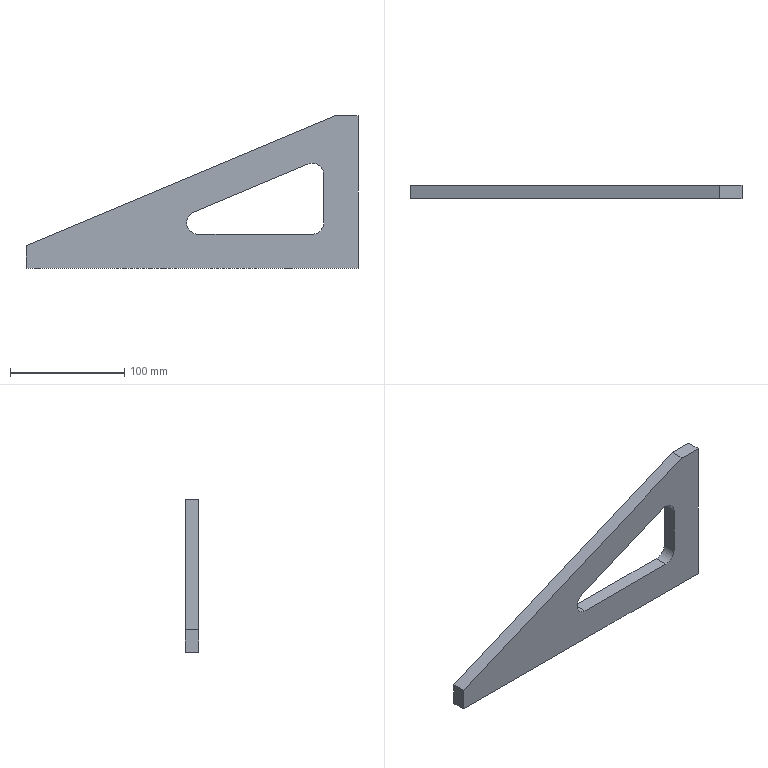Part | SolidWorks | features HoleWzd 2, Extrusion 1, ICE 1 | 1 solid | 34 faces | box 291 x 12 x 134 mm | volume 221726 mm3 | cylinder 14 | cone 10 | plane 10 | commonest cylinder face diameters 5 x10 20 x4
STEP:
#1=CARTESIAN_POINT('',(-133.,0.,-52.));
#2=VERTEX_POINT('',#1);
#3=CARTESIAN_POINT('',(-138.,0.,-52.));
#4=VERTEX_POINT('',#3);
#5=CARTESIAN_POINT('',(-135.5,0.,-52.));
#6=DIRECTION('',(0.,0.,-1.));
#7=DIRECTION('',(-1.,0.,0.));
#8=AXIS2_PLACEMENT_3D('',#5,#6,#7);
#9=CIRCLE('',#8,2.5);
#10=EDGE_CURVE('',#2,#4,#9,.T.);
#11=ORIENTED_EDGE('',*,*,#10,.F.);
#12=CARTESIAN_POINT('',(-133.,0.,-67.));
#13=VERTEX_POINT('',#12);
#14=CARTESIAN_POINT('',(-133.,0.,-67.));
#15=DIRECTION('',(0.,0.,-1.));
#16=VECTOR('',#15,1000.);
#17=LINE('',#14,#16);
#18=EDGE_CURVE('',#2,#13,#17,.T.);
#19=ORIENTED_EDGE('',*,*,#18,.T.);
#20=CARTESIAN_POINT('',(-138.,0.,-67.));
#21=VERTEX_POINT('',#20);
#22=CARTESIAN_POINT('',(-135.5,0.,-67.));
#23=DIRECTION('',(0.,0.,-1.));
#24=DIRECTION('',(-1.,0.,0.));
#25=AXIS2_PLACEMENT_3D('',#22,#23,#24);
#26=CIRCLE('',#25,2.5);
#27=EDGE_CURVE('',#13,#21,#26,.T.);
#28=ORIENTED_EDGE('',*,*,#27,.T.);
#29=CARTESIAN_POINT('',(-138.,0.,-67.));
#30=DIRECTION('',(0.,0.,-1.));
#31=VECTOR('',#30,1000.);
#32=LINE('',#29,#31);
#33=EDGE_CURVE('',#4,#21,#32,.T.);
#34=ORIENTED_EDGE('',*,*,#33,.F.);
#35=EDGE_LOOP('',(#11,#19,#28,#34));
#36=FACE_OUTER_BOUND('',#35,.T.);
#37=CARTESIAN_POINT('',(-135.5,0.,-67.));
#38=DIRECTION('',(0.,0.,-1.));
#39=DIRECTION('',(-1.,0.,0.));
#40=AXIS2_PLACEMENT_3D('',#37,#38,#39);
#41=CYLINDRICAL_SURFACE('',#40,2.5);
#42=ADVANCED_FACE('',(#36),#41,.F.);
#43=CARTESIAN_POINT('',(-135.5,0.,-50.498));
#44=VERTEX_POINT('',#43);
#45=CARTESIAN_POINT('',(-138.,0.,-52.));
#46=DIRECTION('',(-0.8572,0.,-0.515));
#47=VECTOR('',#46,1000.);
#48=LINE('',#45,#47);
#49=EDGE_CURVE('',#44,#4,#48,.T.);
#50=ORIENTED_EDGE('',*,*,#49,.F.);
#51=CARTESIAN_POINT('',(-133.,0.,-52.));
#52=DIRECTION('',(0.8572,0.,-0.515));
#53=VECTOR('',#52,1000.);
#54=LINE('',#51,#53);
#55=EDGE_CURVE('',#44,#2,#54,.T.);
#56=ORIENTED_EDGE('',*,*,#55,.T.);
#57=ORIENTED_EDGE('',*,*,#10,.T.);
#58=EDGE_LOOP('',(#50,#56,#57));
#59=FACE_OUTER_BOUND('',#58,.T.);
#60=CARTESIAN_POINT('',(-135.5,0.,-52.));
#61=DIRECTION('',(0.,0.,-1.));
#62=DIRECTION('',(-1.,0.,0.));
#63=AXIS2_PLACEMENT_3D('',#60,#61,#62);
#64=CONICAL_SURFACE('',#63,2.5,1.03);
#65=ADVANCED_FACE('',(#59),#64,.F.);
#66=CARTESIAN_POINT('',(-23.,0.,-52.));
#67=VERTEX_POINT('',#66);
#68=CARTESIAN_POINT('',(-28.,0.,-52.));
#69=VERTEX_POINT('',#68);
#70=CARTESIAN_POINT('',(-25.5,0.,-52.));
#71=DIRECTION('',(0.,0.,-1.));
#72=DIRECTION('',(-1.,0.,0.));
#73=AXIS2_PLACEMENT_3D('',#70,#71,#72);
#74=CIRCLE('',#73,2.5);
#75=EDGE_CURVE('',#67,#69,#74,.T.);
#76=ORIENTED_EDGE('',*,*,#75,.F.);
#77=CARTESIAN_POINT('',(-23.,0.,-67.));
#78=VERTEX_POINT('',#77);
#79=CARTESIAN_POINT('',(-23.,0.,-67.));
#80=DIRECTION('',(0.,0.,-1.));
#81=VECTOR('',#80,1000.);
#82=LINE('',#79,#81);
#83=EDGE_CURVE('',#67,#78,#82,.T.);
#84=ORIENTED_EDGE('',*,*,#83,.T.);
#85=CARTESIAN_POINT('',(-28.,0.,-67.));
#86=VERTEX_POINT('',#85);
#87=CARTESIAN_POINT('',(-25.5,0.,-67.));
#88=DIRECTION('',(0.,0.,-1.));
#89=DIRECTION('',(-1.,0.,0.));
#90=AXIS2_PLACEMENT_3D('',#87,#88,#89);
#91=CIRCLE('',#90,2.5);
#92=EDGE_CURVE('',#78,#86,#91,.T.);
#93=ORIENTED_EDGE('',*,*,#92,.T.);
#94=CARTESIAN_POINT('',(-28.,0.,-67.));
#95=DIRECTION('',(0.,0.,-1.));
#96=VECTOR('',#95,1000.);
#97=LINE('',#94,#96);
#98=EDGE_CURVE('',#69,#86,#97,.T.);
#99=ORIENTED_EDGE('',*,*,#98,.F.);
#100=EDGE_LOOP('',(#76,#84,#93,#99));
#101=FACE_OUTER_BOUND('',#100,.T.);
#102=CARTESIAN_POINT('',(-25.5,0.,-67.));
#103=DIRECTION('',(0.,0.,-1.));
#104=DIRECTION('',(-1.,0.,0.));
#105=AXIS2_PLACEMENT_3D('',#102,#103,#104);
#106=CYLINDRICAL_SURFACE('',#105,2.5);
#107=ADVANCED_FACE('',(#101),#106,.F.);
#108=CARTESIAN_POINT('',(-25.5,0.,-50.498));
#109=VERTEX_POINT('',#108);
#110=CARTESIAN_POINT('',(-28.,0.,-52.));
#111=DIRECTION('',(-0.8572,0.,-0.515));
#112=VECTOR('',#111,1000.);
#113=LINE('',#110,#112);
#114=EDGE_CURVE('',#109,#69,#113,.T.);
#115=ORIENTED_EDGE('',*,*,#114,.F.);
#116=CARTESIAN_POINT('',(-23.,0.,-52.));
#117=DIRECTION('',(0.8572,0.,-0.515));
#118=VECTOR('',#117,1000.);
#119=LINE('',#116,#118);
#120=EDGE_CURVE('',#109,#67,#119,.T.);
#121=ORIENTED_EDGE('',*,*,#120,.T.);
#122=ORIENTED_EDGE('',*,*,#75,.T.);
#123=EDGE_LOOP('',(#115,#121,#122));
#124=FACE_OUTER_BOUND('',#123,.T.);
#125=CARTESIAN_POINT('',(-25.5,0.,-52.));
#126=DIRECTION('',(0.,0.,-1.));
#127=DIRECTION('',(-1.,0.,0.));
#128=AXIS2_PLACEMENT_3D('',#125,#126,#127);
#129=CONICAL_SURFACE('',#128,2.5,1.03);
#130=ADVANCED_FACE('',(#124),#129,.F.);
#131=CARTESIAN_POINT('',(87.,0.,-52.));
#132=VERTEX_POINT('',#131);
#133=CARTESIAN_POINT('',(82.,0.,-52.));
#134=VERTEX_POINT('',#133);
#135=CARTESIAN_POINT('',(84.5,0.,-52.));
#136=DIRECTION('',(0.,0.,-1.));
#137=DIRECTION('',(-1.,0.,0.));
#138=AXIS2_PLACEMENT_3D('',#135,#136,#137);
#139=CIRCLE('',#138,2.5);
#140=EDGE_CURVE('',#132,#134,#139,.T.);
#141=ORIENTED_EDGE('',*,*,#140,.F.);
#142=CARTESIAN_POINT('',(87.,0.,-67.));
#143=VERTEX_POINT('',#142);
#144=CARTESIAN_POINT('',(87.,0.,-67.));
#145=DIRECTION('',(0.,0.,-1.));
#146=VECTOR('',#145,1000.);
#147=LINE('',#144,#146);
#148=EDGE_CURVE('',#132,#143,#147,.T.);
#149=ORIENTED_EDGE('',*,*,#148,.T.);
#150=CARTESIAN_POINT('',(82.,0.,-67.));
#151=VERTEX_POINT('',#150);
#152=CARTESIAN_POINT('',(84.5,0.,-67.));
#153=DIRECTION('',(0.,0.,-1.));
#154=DIRECTION('',(-1.,0.,0.));
#155=AXIS2_PLACEMENT_3D('',#152,#153,#154);
#156=CIRCLE('',#155,2.5);
#157=EDGE_CURVE('',#143,#151,#156,.T.);
#158=ORIENTED_EDGE('',*,*,#157,.T.);
#159=CARTESIAN_POINT('',(82.,0.,-67.));
#160=DIRECTION('',(0.,0.,-1.));
#161=VECTOR('',#160,1000.);
#162=LINE('',#159,#161);
#163=EDGE_CURVE('',#134,#151,#162,.T.);
#164=ORIENTED_EDGE('',*,*,#163,.F.);
#165=EDGE_LOOP('',(#141,#149,#158,#164));
#166=FACE_OUTER_BOUND('',#165,.T.);
#167=CARTESIAN_POINT('',(84.5,0.,-67.));
#168=DIRECTION('',(0.,0.,-1.));
#169=DIRECTION('',(-1.,0.,0.));
#170=AXIS2_PLACEMENT_3D('',#167,#168,#169);
#171=CYLINDRICAL_SURFACE('',#170,2.5);
#172=ADVANCED_FACE('',(#166),#171,.F.);
#173=CARTESIAN_POINT('',(84.5,0.,-50.498));
#174=VERTEX_POINT('',#173);
#175=CARTESIAN_POINT('',(82.,0.,-52.));
#176=DIRECTION('',(-0.8572,0.,-0.515));
#177=VECTOR('',#176,1000.);
#178=LINE('',#175,#177);
#179=EDGE_CURVE('',#174,#134,#178,.T.);
#180=ORIENTED_EDGE('',*,*,#179,.F.);
#181=CARTESIAN_POINT('',(87.,0.,-52.));
#182=DIRECTION('',(0.8572,0.,-0.515));
#183=VECTOR('',#182,1000.);
#184=LINE('',#181,#183);
#185=EDGE_CURVE('',#174,#132,#184,.T.);
#186=ORIENTED_EDGE('',*,*,#185,.T.);
#187=ORIENTED_EDGE('',*,*,#140,.T.);
#188=EDGE_LOOP('',(#180,#186,#187));
#189=FACE_OUTER_BOUND('',#188,.T.);
#190=CARTESIAN_POINT('',(84.5,0.,-52.));
#191=DIRECTION('',(0.,0.,-1.));
#192=DIRECTION('',(-1.,0.,0.));
#193=AXIS2_PLACEMENT_3D('',#190,#191,#192);
#194=CONICAL_SURFACE('',#193,2.5,1.03);
#195=ADVANCED_FACE('',(#189),#194,.F.);
#196=CARTESIAN_POINT('',(130.5,0.,59.5));
#197=VERTEX_POINT('',#196);
#198=CARTESIAN_POINT('',(130.5,0.,54.5));
#199=VERTEX_POINT('',#198);
#200=CARTESIAN_POINT('',(130.5,0.,57.));
#201=DIRECTION('',(1.,0.,0.));
#202=DIRECTION('',(0.,0.,-1.));
#203=AXIS2_PLACEMENT_3D('',#200,#201,#202);
#204=CIRCLE('',#203,2.5);
#205=EDGE_CURVE('',#197,#199,#204,.T.);
#206=ORIENTED_EDGE('',*,*,#205,.F.);
#207=CARTESIAN_POINT('',(145.5,0.,59.5));
#208=VERTEX_POINT('',#207);
#209=CARTESIAN_POINT('',(145.5,0.,59.5));
#210=DIRECTION('',(1.,0.,0.));
#211=VECTOR('',#210,1000.);
#212=LINE('',#209,#211);
#213=EDGE_CURVE('',#197,#208,#212,.T.);
#214=ORIENTED_EDGE('',*,*,#213,.T.);
#215=CARTESIAN_POINT('',(145.5,0.,54.5));
#216=VERTEX_POINT('',#215);
#217=CARTESIAN_POINT('',(145.5,0.,57.));
#218=DIRECTION('',(1.,0.,0.));
#219=DIRECTION('',(0.,0.,-1.));
#220=AXIS2_PLACEMENT_3D('',#217,#218,#219);
#221=CIRCLE('',#220,2.5);
#222=EDGE_CURVE('',#208,#216,#221,.T.);
#223=ORIENTED_EDGE('',*,*,#222,.T.);
#224=CARTESIAN_POINT('',(145.5,0.,54.5));
#225=DIRECTION('',(1.,0.,0.));
#226=VECTOR('',#225,1000.);
#227=LINE('',#224,#226);
#228=EDGE_CURVE('',#199,#216,#227,.T.);
#229=ORIENTED_EDGE('',*,*,#228,.F.);
#230=EDGE_LOOP('',(#206,#214,#223,#229));
#231=FACE_OUTER_BOUND('',#230,.T.);
#232=CARTESIAN_POINT('',(145.5,0.,57.));
#233=DIRECTION('',(1.,0.,0.));
#234=DIRECTION('',(0.,0.,-1.));
#235=AXIS2_PLACEMENT_3D('',#232,#233,#234);
#236=CYLINDRICAL_SURFACE('',#235,2.5);
#237=ADVANCED_FACE('',(#231),#236,.F.);
#238=CARTESIAN_POINT('',(128.998,0.,57.));
#239=VERTEX_POINT('',#238);
#240=CARTESIAN_POINT('',(130.5,0.,54.5));
#241=DIRECTION('',(0.515,0.,-0.8572));
#242=VECTOR('',#241,1000.);
#243=LINE('',#240,#242);
#244=EDGE_CURVE('',#239,#199,#243,.T.);
#245=ORIENTED_EDGE('',*,*,#244,.F.);
#246=CARTESIAN_POINT('',(130.5,0.,59.5));
#247=DIRECTION('',(0.515,0.,0.8572));
#248=VECTOR('',#247,1000.);
#249=LINE('',#246,#248);
#250=EDGE_CURVE('',#239,#197,#249,.T.);
#251=ORIENTED_EDGE('',*,*,#250,.T.);
#252=ORIENTED_EDGE('',*,*,#205,.T.);
#253=EDGE_LOOP('',(#245,#251,#252));
#254=FACE_OUTER_BOUND('',#253,.T.);
#255=CARTESIAN_POINT('',(130.5,0.,57.));
#256=DIRECTION('',(1.,0.,0.));
#257=DIRECTION('',(0.,0.,-1.));
#258=AXIS2_PLACEMENT_3D('',#255,#256,#257);
#259=CONICAL_SURFACE('',#258,2.5,1.03);
#260=ADVANCED_FACE('',(#254),#259,.F.);
#261=CARTESIAN_POINT('',(130.5,0.,-40.5));
#262=VERTEX_POINT('',#261);
#263=CARTESIAN_POINT('',(130.5,0.,-45.5));
#264=VERTEX_POINT('',#263);
#265=CARTESIAN_POINT('',(130.5,0.,-43.));
#266=DIRECTION('',(1.,0.,0.));
#267=DIRECTION('',(0.,0.,-1.));
#268=AXIS2_PLACEMENT_3D('',#265,#266,#267);
#269=CIRCLE('',#268,2.5);
#270=EDGE_CURVE('',#262,#264,#269,.T.);
#271=ORIENTED_EDGE('',*,*,#270,.F.);
#272=CARTESIAN_POINT('',(145.5,0.,-40.5));
#273=VERTEX_POINT('',#272);
#274=CARTESIAN_POINT('',(145.5,0.,-40.5));
#275=DIRECTION('',(1.,0.,0.));
#276=VECTOR('',#275,1000.);
#277=LINE('',#274,#276);
#278=EDGE_CURVE('',#262,#273,#277,.T.);
#279=ORIENTED_EDGE('',*,*,#278,.T.);
#280=CARTESIAN_POINT('',(145.5,0.,-45.5));
#281=VERTEX_POINT('',#280);
#282=CARTESIAN_POINT('',(145.5,0.,-43.));
#283=DIRECTION('',(1.,0.,0.));
#284=DIRECTION('',(0.,0.,-1.));
#285=AXIS2_PLACEMENT_3D('',#282,#283,#284);
#286=CIRCLE('',#285,2.5);
#287=EDGE_CURVE('',#273,#281,#286,.T.);
#288=ORIENTED_EDGE('',*,*,#287,.T.);
#289=CARTESIAN_POINT('',(145.5,0.,-45.5));
#290=DIRECTION('',(1.,0.,0.));
#291=VECTOR('',#290,1000.);
#292=LINE('',#289,#291);
#293=EDGE_CURVE('',#264,#281,#292,.T.);
#294=ORIENTED_EDGE('',*,*,#293,.F.);
#295=EDGE_LOOP('',(#271,#279,#288,#294));
#296=FACE_OUTER_BOUND('',#295,.T.);
#297=CARTESIAN_POINT('',(145.5,0.,-43.));
#298=DIRECTION('',(1.,0.,0.));
#299=DIRECTION('',(0.,0.,-1.));
#300=AXIS2_PLACEMENT_3D('',#297,#298,#299);
#301=CYLINDRICAL_SURFACE('',#300,2.5);
#302=ADVANCED_FACE('',(#296),#301,.F.);
#303=CARTESIAN_POINT('',(128.998,0.,-43.));
#304=VERTEX_POINT('',#303);
#305=CARTESIAN_POINT('',(130.5,0.,-45.5));
#306=DIRECTION('',(0.515,0.,-0.8572));
#307=VECTOR('',#306,1000.);
#308=LINE('',#305,#307);
#309=EDGE_CURVE('',#304,#264,#308,.T.);
#310=ORIENTED_EDGE('',*,*,#309,.F.);
#311=CARTESIAN_POINT('',(130.5,0.,-40.5));
#312=DIRECTION('',(0.515,0.,0.8572));
#313=VECTOR('',#312,1000.);
#314=LINE('',#311,#313);
#315=EDGE_CURVE('',#304,#262,#314,.T.);
#316=ORIENTED_EDGE('',*,*,#315,.T.);
#317=ORIENTED_EDGE('',*,*,#270,.T.);
#318=EDGE_LOOP('',(#310,#316,#317));
#319=FACE_OUTER_BOUND('',#318,.T.);
#320=CARTESIAN_POINT('',(130.5,0.,-43.));
#321=DIRECTION('',(1.,0.,0.));
#322=DIRECTION('',(0.,0.,-1.));
#323=AXIS2_PLACEMENT_3D('',#320,#321,#322);
#324=CONICAL_SURFACE('',#323,2.5,1.03);
#325=ADVANCED_FACE('',(#319),#324,.F.);
#326=CARTESIAN_POINT('',(105.5,-6.,25.192));
#327=VERTEX_POINT('',#326);
#328=CARTESIAN_POINT('',(115.5,-6.,15.192));
#329=VERTEX_POINT('',#328);
#330=CARTESIAN_POINT('',(105.5,-6.,15.192));
#331=DIRECTION('',(0.,1.,0.));
#332=DIRECTION('',(0.,0.,-1.));
#333=AXIS2_PLACEMENT_3D('',#330,#331,#332);
#334=CIRCLE('',#333,10.);
#335=EDGE_CURVE('',#327,#329,#334,.T.);
#336=ORIENTED_EDGE('',*,*,#335,.F.);
#337=CARTESIAN_POINT('',(105.5,6.,25.192));
#338=VERTEX_POINT('',#337);
#339=CARTESIAN_POINT('',(105.5,-6.,25.192));
#340=DIRECTION('',(0.,1.,0.));
#341=VECTOR('',#340,1000.);
#342=LINE('',#339,#341);
#343=EDGE_CURVE('',#327,#338,#342,.T.);
#344=ORIENTED_EDGE('',*,*,#343,.T.);
#345=CARTESIAN_POINT('',(115.5,6.,15.192));
#346=VERTEX_POINT('',#345);
#347=CARTESIAN_POINT('',(105.5,6.,15.192));
#348=DIRECTION('',(0.,1.,0.));
#349=DIRECTION('',(0.,0.,-1.));
#350=AXIS2_PLACEMENT_3D('',#347,#348,#349);
#351=CIRCLE('',#350,10.);
#352=EDGE_CURVE('',#338,#346,#351,.T.);
#353=ORIENTED_EDGE('',*,*,#352,.T.);
#354=CARTESIAN_POINT('',(115.5,-6.,15.192));
#355=DIRECTION('',(0.,1.,0.));
#356=VECTOR('',#355,1000.);
#357=LINE('',#354,#356);
#358=EDGE_CURVE('',#329,#346,#357,.T.);
#359=ORIENTED_EDGE('',*,*,#358,.F.);
#360=EDGE_LOOP('',(#336,#344,#353,#359));
#361=FACE_OUTER_BOUND('',#360,.T.);
#362=CARTESIAN_POINT('',(105.5,-6.,15.192));
#363=DIRECTION('',(0.,1.,0.));
#364=DIRECTION('',(0.,0.,1.));
#365=AXIS2_PLACEMENT_3D('',#362,#363,#364);
#366=CYLINDRICAL_SURFACE('',#365,10.);
#367=ADVANCED_FACE('',(#361),#366,.F.);
#368=CARTESIAN_POINT('',(145.5,0.,57.));
#369=DIRECTION('',(1.,0.,0.));
#370=DIRECTION('',(0.,0.,-1.));
#371=AXIS2_PLACEMENT_3D('',#368,#369,#370);
#372=CIRCLE('',#371,2.5);
#373=EDGE_CURVE('',#216,#208,#372,.T.);
#374=ORIENTED_EDGE('',*,*,#373,.F.);
#375=ORIENTED_EDGE('',*,*,#222,.F.);
#376=EDGE_LOOP('',(#374,#375));
#377=FACE_BOUND('',#376,.T.);
#378=CARTESIAN_POINT('',(145.5,0.,-43.));
#379=DIRECTION('',(1.,0.,0.));
#380=DIRECTION('',(0.,0.,-1.));
#381=AXIS2_PLACEMENT_3D('',#378,#379,#380);
#382=CIRCLE('',#381,2.5);
#383=EDGE_CURVE('',#281,#273,#382,.T.);
#384=ORIENTED_EDGE('',*,*,#383,.F.);
#385=ORIENTED_EDGE('',*,*,#287,.F.);
#386=EDGE_LOOP('',(#384,#385));
#387=FACE_BOUND('',#386,.T.);
#388=CARTESIAN_POINT('',(145.5,-6.,67.));
#389=VERTEX_POINT('',#388);
#390=CARTESIAN_POINT('',(145.5,-6.,-67.));
#391=VERTEX_POINT('',#390);
#392=CARTESIAN_POINT('',(145.5,-6.,67.));
#393=DIRECTION('',(0.,0.,-1.));
#394=VECTOR('',#393,1000.);
#395=LINE('',#392,#394);
#396=EDGE_CURVE('',#389,#391,#395,.T.);
#397=ORIENTED_EDGE('',*,*,#396,.T.);
#398=CARTESIAN_POINT('',(145.5,6.,-67.));
#399=VERTEX_POINT('',#398);
#400=CARTESIAN_POINT('',(145.5,6.,-67.));
#401=DIRECTION('',(0.,-1.,0.));
#402=VECTOR('',#401,1000.);
#403=LINE('',#400,#402);
#404=EDGE_CURVE('',#399,#391,#403,.T.);
#405=ORIENTED_EDGE('',*,*,#404,.F.);
#406=CARTESIAN_POINT('',(145.5,6.,67.));
#407=VERTEX_POINT('',#406);
#408=CARTESIAN_POINT('',(145.5,6.,67.));
#409=DIRECTION('',(0.,0.,-1.));
#410=VECTOR('',#409,1000.);
#411=LINE('',#408,#410);
#412=EDGE_CURVE('',#407,#399,#411,.T.);
#413=ORIENTED_EDGE('',*,*,#412,.F.);
#414=CARTESIAN_POINT('',(145.5,6.,67.));
#415=DIRECTION('',(0.,-1.,0.));
#416=VECTOR('',#415,1000.);
#417=LINE('',#414,#416);
#418=EDGE_CURVE('',#407,#389,#417,.T.);
#419=ORIENTED_EDGE('',*,*,#418,.T.);
#420=EDGE_LOOP('',(#397,#405,#413,#419));
#421=FACE_OUTER_BOUND('',#420,.T.);
#422=CARTESIAN_POINT('',(145.5,6.,67.));
#423=DIRECTION('',(-1.,0.,0.));
#424=DIRECTION('',(0.,0.,1.));
#425=AXIS2_PLACEMENT_3D('',#422,#423,#424);
#426=PLANE('',#425);
#427=ADVANCED_FACE('',(#377,#387,#421),#426,.F.);
#428=CARTESIAN_POINT('',(-135.5,0.,-67.));
#429=DIRECTION('',(0.,0.,-1.));
#430=DIRECTION('',(-1.,0.,0.));
#431=AXIS2_PLACEMENT_3D('',#428,#429,#430);
#432=CIRCLE('',#431,2.5);
#433=EDGE_CURVE('',#21,#13,#432,.T.);
#434=ORIENTED_EDGE('',*,*,#433,.F.);
#435=ORIENTED_EDGE('',*,*,#27,.F.);
#436=EDGE_LOOP('',(#434,#435));
#437=FACE_BOUND('',#436,.T.);
#438=CARTESIAN_POINT('',(-25.5,0.,-67.));
#439=DIRECTION('',(0.,0.,-1.));
#440=DIRECTION('',(-1.,0.,0.));
#441=AXIS2_PLACEMENT_3D('',#438,#439,#440);
#442=CIRCLE('',#441,2.5);
#443=EDGE_CURVE('',#86,#78,#442,.T.);
#444=ORIENTED_EDGE('',*,*,#443,.F.);
#445=ORIENTED_EDGE('',*,*,#92,.F.);
#446=EDGE_LOOP('',(#444,#445));
#447=FACE_BOUND('',#446,.T.);
#448=CARTESIAN_POINT('',(84.5,0.,-67.));
#449=DIRECTION('',(0.,0.,-1.));
#450=DIRECTION('',(-1.,0.,0.));
#451=AXIS2_PLACEMENT_3D('',#448,#449,#450);
#452=CIRCLE('',#451,2.5);
#453=EDGE_CURVE('',#151,#143,#452,.T.);
#454=ORIENTED_EDGE('',*,*,#453,.F.);
#455=ORIENTED_EDGE('',*,*,#157,.F.);
#456=EDGE_LOOP('',(#454,#455));
#457=FACE_BOUND('',#456,.T.);
#458=CARTESIAN_POINT('',(-145.5,-6.,-67.));
#459=VERTEX_POINT('',#458);
#460=CARTESIAN_POINT('',(-145.5,-6.,-67.));
#461=DIRECTION('',(-1.,0.,0.));
#462=VECTOR('',#461,1000.);
#463=LINE('',#460,#462);
#464=EDGE_CURVE('',#391,#459,#463,.T.);
#465=ORIENTED_EDGE('',*,*,#464,.T.);
#466=CARTESIAN_POINT('',(-145.5,6.,-67.));
#467=VERTEX_POINT('',#466);
#468=CARTESIAN_POINT('',(-145.5,6.,-67.));
#469=DIRECTION('',(0.,-1.,0.));
#470=VECTOR('',#469,1000.);
#471=LINE('',#468,#470);
#472=EDGE_CURVE('',#467,#459,#471,.T.);
#473=ORIENTED_EDGE('',*,*,#472,.F.);
#474=CARTESIAN_POINT('',(-145.5,6.,-67.));
#475=DIRECTION('',(-1.,0.,0.));
#476=VECTOR('',#475,1000.);
#477=LINE('',#474,#476);
#478=EDGE_CURVE('',#399,#467,#477,.T.);
#479=ORIENTED_EDGE('',*,*,#478,.F.);
#480=ORIENTED_EDGE('',*,*,#404,.T.);
#481=EDGE_LOOP('',(#465,#473,#479,#480));
#482=FACE_OUTER_BOUND('',#481,.T.);
#483=CARTESIAN_POINT('',(-145.5,6.,-67.));
#484=DIRECTION('',(0.,0.,1.));
#485=DIRECTION('',(1.,0.,0.));
#486=AXIS2_PLACEMENT_3D('',#483,#484,#485);
#487=PLANE('',#486);
#488=ADVANCED_FACE('',(#437,#447,#457,#482),#487,.F.);
#489=CARTESIAN_POINT('',(-145.5,-6.,-47.));
#490=VERTEX_POINT('',#489);
#491=CARTESIAN_POINT('',(-145.5,-6.,67.));
#492=DIRECTION('',(0.,0.,1.));
#493=VECTOR('',#492,1000.);
#494=LINE('',#491,#493);
#495=EDGE_CURVE('',#459,#490,#494,.T.);
#496=ORIENTED_EDGE('',*,*,#495,.T.);
#497=CARTESIAN_POINT('',(-145.5,6.,-47.));
#498=VERTEX_POINT('',#497);
#499=CARTESIAN_POINT('',(-145.5,-6.,-47.));
#500=DIRECTION('',(0.,1.,0.));
#501=VECTOR('',#500,1000.);
#502=LINE('',#499,#501);
#503=EDGE_CURVE('',#490,#498,#502,.T.);
#504=ORIENTED_EDGE('',*,*,#503,.T.);
#505=CARTESIAN_POINT('',(-145.5,6.,67.));
#506=DIRECTION('',(0.,0.,1.));
#507=VECTOR('',#506,1000.);
#508=LINE('',#505,#507);
#509=EDGE_CURVE('',#467,#498,#508,.T.);
#510=ORIENTED_EDGE('',*,*,#509,.F.);
#511=ORIENTED_EDGE('',*,*,#472,.T.);
#512=EDGE_LOOP('',(#496,#504,#510,#511));
#513=FACE_OUTER_BOUND('',#512,.T.);
#514=CARTESIAN_POINT('',(-145.5,6.,67.));
#515=DIRECTION('',(1.,0.,0.));
#516=DIRECTION('',(0.,0.,-1.));
#517=AXIS2_PLACEMENT_3D('',#514,#515,#516);
#518=PLANE('',#517);
#519=ADVANCED_FACE('',(#513),#518,.F.);
#520=CARTESIAN_POINT('',(125.5,6.,67.));
#521=VERTEX_POINT('',#520);
#522=CARTESIAN_POINT('',(-145.5,6.,67.));
#523=DIRECTION('',(1.,0.,0.));
#524=VECTOR('',#523,1000.);
#525=LINE('',#522,#524);
#526=EDGE_CURVE('',#521,#407,#525,.T.);
#527=ORIENTED_EDGE('',*,*,#526,.F.);
#528=CARTESIAN_POINT('',(125.5,-6.,67.));
#529=VERTEX_POINT('',#528);
#530=CARTESIAN_POINT('',(125.5,-6.,67.));
#531=DIRECTION('',(0.,1.,0.));
#532=VECTOR('',#531,1000.);
#533=LINE('',#530,#532);
#534=EDGE_CURVE('',#529,#521,#533,.T.);
#535=ORIENTED_EDGE('',*,*,#534,.F.);
#536=CARTESIAN_POINT('',(-145.5,-6.,67.));
#537=DIRECTION('',(1.,0.,0.));
#538=VECTOR('',#537,1000.);
#539=LINE('',#536,#538);
#540=EDGE_CURVE('',#529,#389,#539,.T.);
#541=ORIENTED_EDGE('',*,*,#540,.T.);
#542=ORIENTED_EDGE('',*,*,#418,.F.);
#543=EDGE_LOOP('',(#527,#535,#541,#542));
#544=FACE_OUTER_BOUND('',#543,.T.);
#545=CARTESIAN_POINT('',(-145.5,6.,67.));
#546=DIRECTION('',(0.,0.,-1.));
#547=DIRECTION('',(-1.,0.,0.));
#548=AXIS2_PLACEMENT_3D('',#545,#546,#547);
#549=PLANE('',#548);
#550=ADVANCED_FACE('',(#544),#549,.F.);
#551=CARTESIAN_POINT('',(1.325,6.,-17.782));
#552=VERTEX_POINT('',#551);
#553=CARTESIAN_POINT('',(101.622,6.,24.409));
#554=VERTEX_POINT('',#553);
#555=CARTESIAN_POINT('',(1.325,6.,-17.782));
#556=DIRECTION('',(0.9218,0.,0.3878));
#557=VECTOR('',#556,1000.);
#558=LINE('',#555,#557);
#559=EDGE_CURVE('',#552,#554,#558,.T.);
#560=ORIENTED_EDGE('',*,*,#559,.F.);
#561=CARTESIAN_POINT('',(5.202,6.,-37.));
#562=VERTEX_POINT('',#561);
#563=CARTESIAN_POINT('',(5.202,6.,-27.));
#564=DIRECTION('',(0.,1.,0.));
#565=DIRECTION('',(0.,0.,1.));
#566=AXIS2_PLACEMENT_3D('',#563,#564,#565);
#567=CIRCLE('',#566,10.);
#568=EDGE_CURVE('',#562,#552,#567,.T.);
#569=ORIENTED_EDGE('',*,*,#568,.F.);
#570=CARTESIAN_POINT('',(105.5,6.,-37.));
#571=VERTEX_POINT('',#570);
#572=CARTESIAN_POINT('',(105.5,6.,-37.));
#573=DIRECTION('',(-1.,0.,0.));
#574=VECTOR('',#573,1000.);
#575=LINE('',#572,#574);
#576=EDGE_CURVE('',#571,#562,#575,.T.);
#577=ORIENTED_EDGE('',*,*,#576,.F.);
#578=CARTESIAN_POINT('',(115.5,6.,-27.));
#579=VERTEX_POINT('',#578);
#580=CARTESIAN_POINT('',(105.5,6.,-27.));
#581=DIRECTION('',(0.,1.,0.));
#582=DIRECTION('',(0.,0.,1.));
#583=AXIS2_PLACEMENT_3D('',#580,#581,#582);
#584=CIRCLE('',#583,10.);
#585=EDGE_CURVE('',#579,#571,#584,.T.);
#586=ORIENTED_EDGE('',*,*,#585,.F.);
#587=CARTESIAN_POINT('',(115.5,6.,15.192));
#588=DIRECTION('',(0.,0.,-1.));
#589=VECTOR('',#588,1000.);
#590=LINE('',#587,#589);
#591=EDGE_CURVE('',#346,#579,#590,.T.);
#592=ORIENTED_EDGE('',*,*,#591,.F.);
#593=ORIENTED_EDGE('',*,*,#352,.F.);
#594=CARTESIAN_POINT('',(105.5,6.,15.192));
#595=DIRECTION('',(0.,1.,0.));
#596=DIRECTION('',(0.,0.,-1.));
#597=AXIS2_PLACEMENT_3D('',#594,#595,#596);
#598=CIRCLE('',#597,10.);
#599=EDGE_CURVE('',#554,#338,#598,.T.);
#600=ORIENTED_EDGE('',*,*,#599,.F.);
#601=EDGE_LOOP('',(#560,#569,#577,#586,#592,#593,#600));
#602=FACE_BOUND('',#601,.T.);
#603=ORIENTED_EDGE('',*,*,#509,.T.);
#604=CARTESIAN_POINT('',(-145.5,6.,-47.));
#605=DIRECTION('',(-0.9218,0.,-0.3878));
#606=VECTOR('',#605,1000.);
#607=LINE('',#604,#606);
#608=EDGE_CURVE('',#521,#498,#607,.T.);
#609=ORIENTED_EDGE('',*,*,#608,.F.);
#610=ORIENTED_EDGE('',*,*,#526,.T.);
#611=ORIENTED_EDGE('',*,*,#412,.T.);
#612=ORIENTED_EDGE('',*,*,#478,.T.);
#613=EDGE_LOOP('',(#603,#609,#610,#611,#612));
#614=FACE_OUTER_BOUND('',#613,.T.);
#615=CARTESIAN_POINT('',(0.,6.,0.));
#616=DIRECTION('',(0.,-1.,0.));
#617=DIRECTION('',(0.,0.,-1.));
#618=AXIS2_PLACEMENT_3D('',#615,#616,#617);
#619=PLANE('',#618);
#620=ADVANCED_FACE('',(#602,#614),#619,.F.);
#621=CARTESIAN_POINT('',(5.202,-6.,-37.));
#622=VERTEX_POINT('',#621);
#623=CARTESIAN_POINT('',(1.325,-6.,-17.782));
#624=VERTEX_POINT('',#623);
#625=CARTESIAN_POINT('',(5.202,-6.,-27.));
#626=DIRECTION('',(0.,1.,0.));
#627=DIRECTION('',(0.,0.,1.));
#628=AXIS2_PLACEMENT_3D('',#625,#626,#627);
#629=CIRCLE('',#628,10.);
#630=EDGE_CURVE('',#622,#624,#629,.T.);
#631=ORIENTED_EDGE('',*,*,#630,.T.);
#632=CARTESIAN_POINT('',(101.622,-6.,24.409));
#633=VERTEX_POINT('',#632);
#634=CARTESIAN_POINT('',(1.325,-6.,-17.782));
#635=DIRECTION('',(0.9218,0.,0.3878));
#636=VECTOR('',#635,1000.);
#637=LINE('',#634,#636);
#638=EDGE_CURVE('',#624,#633,#637,.T.);
#639=ORIENTED_EDGE('',*,*,#638,.T.);
#640=CARTESIAN_POINT('',(105.5,-6.,15.192));
#641=DIRECTION('',(0.,1.,0.));
#642=DIRECTION('',(0.,0.,-1.));
#643=AXIS2_PLACEMENT_3D('',#640,#641,#642);
#644=CIRCLE('',#643,10.);
#645=EDGE_CURVE('',#633,#327,#644,.T.);
#646=ORIENTED_EDGE('',*,*,#645,.T.);
#647=ORIENTED_EDGE('',*,*,#335,.T.);
#648=CARTESIAN_POINT('',(115.5,-6.,-27.));
#649=VERTEX_POINT('',#648);
#650=CARTESIAN_POINT('',(115.5,-6.,15.192));
#651=DIRECTION('',(0.,0.,-1.));
#652=VECTOR('',#651,1000.);
#653=LINE('',#650,#652);
#654=EDGE_CURVE('',#329,#649,#653,.T.);
#655=ORIENTED_EDGE('',*,*,#654,.T.);
#656=CARTESIAN_POINT('',(105.5,-6.,-37.));
#657=VERTEX_POINT('',#656);
#658=CARTESIAN_POINT('',(105.5,-6.,-27.));
#659=DIRECTION('',(0.,1.,0.));
#660=DIRECTION('',(0.,0.,1.));
#661=AXIS2_PLACEMENT_3D('',#658,#659,#660);
#662=CIRCLE('',#661,10.);
#663=EDGE_CURVE('',#649,#657,#662,.T.);
#664=ORIENTED_EDGE('',*,*,#663,.T.);
#665=CARTESIAN_POINT('',(105.5,-6.,-37.));
#666=DIRECTION('',(-1.,0.,0.));
#667=VECTOR('',#666,1000.);
#668=LINE('',#665,#667);
#669=EDGE_CURVE('',#657,#622,#668,.T.);
#670=ORIENTED_EDGE('',*,*,#669,.T.);
#671=EDGE_LOOP('',(#631,#639,#646,#647,#655,#664,#670));
#672=FACE_BOUND('',#671,.T.);
#673=CARTESIAN_POINT('',(-145.5,-6.,-47.));
#674=DIRECTION('',(-0.9218,0.,-0.3878));
#675=VECTOR('',#674,1000.);
#676=LINE('',#673,#675);
#677=EDGE_CURVE('',#529,#490,#676,.T.);
#678=ORIENTED_EDGE('',*,*,#677,.T.);
#679=ORIENTED_EDGE('',*,*,#495,.F.);
#680=ORIENTED_EDGE('',*,*,#464,.F.);
#681=ORIENTED_EDGE('',*,*,#396,.F.);
#682=ORIENTED_EDGE('',*,*,#540,.F.);
#683=EDGE_LOOP('',(#678,#679,#680,#681,#682));
#684=FACE_OUTER_BOUND('',#683,.T.);
#685=CARTESIAN_POINT('',(0.,-6.,0.));
#686=DIRECTION('',(0.,-1.,0.));
#687=DIRECTION('',(0.,0.,-1.));
#688=AXIS2_PLACEMENT_3D('',#685,#686,#687);
#689=PLANE('',#688);
#690=ADVANCED_FACE('',(#672,#684),#689,.T.);
#691=ORIENTED_EDGE('',*,*,#608,.T.);
#692=ORIENTED_EDGE('',*,*,#503,.F.);
#693=ORIENTED_EDGE('',*,*,#677,.F.);
#694=ORIENTED_EDGE('',*,*,#534,.T.);
#695=EDGE_LOOP('',(#691,#692,#693,#694));
#696=FACE_OUTER_BOUND('',#695,.T.);
#697=CARTESIAN_POINT('',(-145.5,-6.,-47.));
#698=DIRECTION('',(0.3878,0.,-0.9218));
#699=DIRECTION('',(-0.9218,0.,-0.3878));
#700=AXIS2_PLACEMENT_3D('',#697,#698,#699);
#701=PLANE('',#700);
#702=ADVANCED_FACE('',(#696),#701,.F.);
#703=ORIENTED_EDGE('',*,*,#568,.T.);
#704=CARTESIAN_POINT('',(1.325,-6.,-17.782));
#705=DIRECTION('',(0.,1.,0.));
#706=VECTOR('',#705,1000.);
#707=LINE('',#704,#706);
#708=EDGE_CURVE('',#624,#552,#707,.T.);
#709=ORIENTED_EDGE('',*,*,#708,.F.);
#710=ORIENTED_EDGE('',*,*,#630,.F.);
#711=CARTESIAN_POINT('',(5.202,-6.,-37.));
#712=DIRECTION('',(0.,1.,0.));
#713=VECTOR('',#712,1000.);
#714=LINE('',#711,#713);
#715=EDGE_CURVE('',#622,#562,#714,.T.);
#716=ORIENTED_EDGE('',*,*,#715,.T.);
#717=EDGE_LOOP('',(#703,#709,#710,#716));
#718=FACE_OUTER_BOUND('',#717,.T.);
#719=CARTESIAN_POINT('',(5.202,-6.,-27.));
#720=DIRECTION('',(0.,1.,0.));
#721=DIRECTION('',(0.,0.,1.));
#722=AXIS2_PLACEMENT_3D('',#719,#720,#721);
#723=CYLINDRICAL_SURFACE('',#722,10.);
#724=ADVANCED_FACE('',(#718),#723,.F.);
#725=ORIENTED_EDGE('',*,*,#576,.T.);
#726=ORIENTED_EDGE('',*,*,#715,.F.);
#727=ORIENTED_EDGE('',*,*,#669,.F.);
#728=CARTESIAN_POINT('',(105.5,-6.,-37.));
#729=DIRECTION('',(0.,1.,0.));
#730=VECTOR('',#729,1000.);
#731=LINE('',#728,#730);
#732=EDGE_CURVE('',#657,#571,#731,.T.);
#733=ORIENTED_EDGE('',*,*,#732,.T.);
#734=EDGE_LOOP('',(#725,#726,#727,#733));
#735=FACE_OUTER_BOUND('',#734,.T.);
#736=CARTESIAN_POINT('',(105.5,-6.,-37.));
#737=DIRECTION('',(0.,0.,-1.));
#738=DIRECTION('',(-1.,0.,0.));
#739=AXIS2_PLACEMENT_3D('',#736,#737,#738);
#740=PLANE('',#739);
#741=ADVANCED_FACE('',(#735),#740,.F.);
#742=ORIENTED_EDGE('',*,*,#585,.T.);
#743=ORIENTED_EDGE('',*,*,#732,.F.);
#744=ORIENTED_EDGE('',*,*,#663,.F.);
#745=CARTESIAN_POINT('',(115.5,-6.,-27.));
#746=DIRECTION('',(0.,1.,0.));
#747=VECTOR('',#746,1000.);
#748=LINE('',#745,#747);
#749=EDGE_CURVE('',#649,#579,#748,.T.);
#750=ORIENTED_EDGE('',*,*,#749,.T.);
#751=EDGE_LOOP('',(#742,#743,#744,#750));
#752=FACE_OUTER_BOUND('',#751,.T.);
#753=CARTESIAN_POINT('',(105.5,-6.,-27.));
#754=DIRECTION('',(0.,1.,0.));
#755=DIRECTION('',(0.,0.,1.));
#756=AXIS2_PLACEMENT_3D('',#753,#754,#755);
#757=CYLINDRICAL_SURFACE('',#756,10.);
#758=ADVANCED_FACE('',(#752),#757,.F.);
#759=ORIENTED_EDGE('',*,*,#591,.T.);
#760=ORIENTED_EDGE('',*,*,#749,.F.);
#761=ORIENTED_EDGE('',*,*,#654,.F.);
#762=ORIENTED_EDGE('',*,*,#358,.T.);
#763=EDGE_LOOP('',(#759,#760,#761,#762));
#764=FACE_OUTER_BOUND('',#763,.T.);
#765=CARTESIAN_POINT('',(115.5,-6.,15.192));
#766=DIRECTION('',(1.,0.,0.));
#767=DIRECTION('',(0.,0.,-1.));
#768=AXIS2_PLACEMENT_3D('',#765,#766,#767);
#769=PLANE('',#768);
#770=ADVANCED_FACE('',(#764),#769,.F.);
#771=ORIENTED_EDGE('',*,*,#343,.F.);
#772=ORIENTED_EDGE('',*,*,#645,.F.);
#773=CARTESIAN_POINT('',(101.622,-6.,24.409));
#774=DIRECTION('',(0.,1.,0.));
#775=VECTOR('',#774,1000.);
#776=LINE('',#773,#775);
#777=EDGE_CURVE('',#633,#554,#776,.T.);
#778=ORIENTED_EDGE('',*,*,#777,.T.);
#779=ORIENTED_EDGE('',*,*,#599,.T.);
#780=EDGE_LOOP('',(#771,#772,#778,#779));
#781=FACE_OUTER_BOUND('',#780,.T.);
#782=CARTESIAN_POINT('',(105.5,-6.,15.192));
#783=DIRECTION('',(0.,1.,0.));
#784=DIRECTION('',(0.,0.,1.));
#785=AXIS2_PLACEMENT_3D('',#782,#783,#784);
#786=CYLINDRICAL_SURFACE('',#785,10.);
#787=ADVANCED_FACE('',(#781),#786,.F.);
#788=ORIENTED_EDGE('',*,*,#559,.T.);
#789=ORIENTED_EDGE('',*,*,#777,.F.);
#790=ORIENTED_EDGE('',*,*,#638,.F.);
#791=ORIENTED_EDGE('',*,*,#708,.T.);
#792=EDGE_LOOP('',(#788,#789,#790,#791));
#793=FACE_OUTER_BOUND('',#792,.T.);
#794=CARTESIAN_POINT('',(1.325,-6.,-17.782));
#795=DIRECTION('',(-0.3878,0.,0.9218));
#796=DIRECTION('',(0.9218,0.,0.3878));
#797=AXIS2_PLACEMENT_3D('',#794,#795,#796);
#798=PLANE('',#797);
#799=ADVANCED_FACE('',(#793),#798,.F.);
#800=ORIENTED_EDGE('',*,*,#315,.F.);
#801=ORIENTED_EDGE('',*,*,#309,.T.);
#802=CARTESIAN_POINT('',(130.5,0.,-43.));
#803=DIRECTION('',(1.,0.,0.));
#804=DIRECTION('',(0.,0.,-1.));
#805=AXIS2_PLACEMENT_3D('',#802,#803,#804);
#806=CIRCLE('',#805,2.5);
#807=EDGE_CURVE('',#264,#262,#806,.T.);
#808=ORIENTED_EDGE('',*,*,#807,.T.);
#809=EDGE_LOOP('',(#800,#801,#808));
#810=FACE_OUTER_BOUND('',#809,.T.);
#811=CARTESIAN_POINT('',(130.5,0.,-43.));
#812=DIRECTION('',(1.,0.,0.));
#813=DIRECTION('',(0.,0.,-1.));
#814=AXIS2_PLACEMENT_3D('',#811,#812,#813);
#815=CONICAL_SURFACE('',#814,2.5,1.03);
#816=ADVANCED_FACE('',(#810),#815,.F.);
#817=ORIENTED_EDGE('',*,*,#278,.F.);
#818=ORIENTED_EDGE('',*,*,#807,.F.);
#819=ORIENTED_EDGE('',*,*,#293,.T.);
#820=ORIENTED_EDGE('',*,*,#383,.T.);
#821=EDGE_LOOP('',(#817,#818,#819,#820));
#822=FACE_OUTER_BOUND('',#821,.T.);
#823=CARTESIAN_POINT('',(145.5,0.,-43.));
#824=DIRECTION('',(1.,0.,0.));
#825=DIRECTION('',(0.,0.,-1.));
#826=AXIS2_PLACEMENT_3D('',#823,#824,#825);
#827=CYLINDRICAL_SURFACE('',#826,2.5);
#828=ADVANCED_FACE('',(#822),#827,.F.);
#829=ORIENTED_EDGE('',*,*,#250,.F.);
#830=ORIENTED_EDGE('',*,*,#244,.T.);
#831=CARTESIAN_POINT('',(130.5,0.,57.));
#832=DIRECTION('',(1.,0.,0.));
#833=DIRECTION('',(0.,0.,-1.));
#834=AXIS2_PLACEMENT_3D('',#831,#832,#833);
#835=CIRCLE('',#834,2.5);
#836=EDGE_CURVE('',#199,#197,#835,.T.);
#837=ORIENTED_EDGE('',*,*,#836,.T.);
#838=EDGE_LOOP('',(#829,#830,#837));
#839=FACE_OUTER_BOUND('',#838,.T.);
#840=CARTESIAN_POINT('',(130.5,0.,57.));
#841=DIRECTION('',(1.,0.,0.));
#842=DIRECTION('',(0.,0.,-1.));
#843=AXIS2_PLACEMENT_3D('',#840,#841,#842);
#844=CONICAL_SURFACE('',#843,2.5,1.03);
#845=ADVANCED_FACE('',(#839),#844,.F.);
#846=ORIENTED_EDGE('',*,*,#213,.F.);
#847=ORIENTED_EDGE('',*,*,#836,.F.);
#848=ORIENTED_EDGE('',*,*,#228,.T.);
#849=ORIENTED_EDGE('',*,*,#373,.T.);
#850=EDGE_LOOP('',(#846,#847,#848,#849));
#851=FACE_OUTER_BOUND('',#850,.T.);
#852=CARTESIAN_POINT('',(145.5,0.,57.));
#853=DIRECTION('',(1.,0.,0.));
#854=DIRECTION('',(0.,0.,-1.));
#855=AXIS2_PLACEMENT_3D('',#852,#853,#854);
#856=CYLINDRICAL_SURFACE('',#855,2.5);
#857=ADVANCED_FACE('',(#851),#856,.F.);
#858=ORIENTED_EDGE('',*,*,#185,.F.);
#859=ORIENTED_EDGE('',*,*,#179,.T.);
#860=CARTESIAN_POINT('',(84.5,0.,-52.));
#861=DIRECTION('',(0.,0.,-1.));
#862=DIRECTION('',(-1.,0.,0.));
#863=AXIS2_PLACEMENT_3D('',#860,#861,#862);
#864=CIRCLE('',#863,2.5);
#865=EDGE_CURVE('',#134,#132,#864,.T.);
#866=ORIENTED_EDGE('',*,*,#865,.T.);
#867=EDGE_LOOP('',(#858,#859,#866));
#868=FACE_OUTER_BOUND('',#867,.T.);
#869=CARTESIAN_POINT('',(84.5,0.,-52.));
#870=DIRECTION('',(0.,0.,-1.));
#871=DIRECTION('',(-1.,0.,0.));
#872=AXIS2_PLACEMENT_3D('',#869,#870,#871);
#873=CONICAL_SURFACE('',#872,2.5,1.03);
#874=ADVANCED_FACE('',(#868),#873,.F.);
#875=ORIENTED_EDGE('',*,*,#148,.F.);
#876=ORIENTED_EDGE('',*,*,#865,.F.);
#877=ORIENTED_EDGE('',*,*,#163,.T.);
#878=ORIENTED_EDGE('',*,*,#453,.T.);
#879=EDGE_LOOP('',(#875,#876,#877,#878));
#880=FACE_OUTER_BOUND('',#879,.T.);
#881=CARTESIAN_POINT('',(84.5,0.,-67.));
#882=DIRECTION('',(0.,0.,-1.));
#883=DIRECTION('',(-1.,0.,0.));
#884=AXIS2_PLACEMENT_3D('',#881,#882,#883);
#885=CYLINDRICAL_SURFACE('',#884,2.5);
#886=ADVANCED_FACE('',(#880),#885,.F.);
#887=ORIENTED_EDGE('',*,*,#120,.F.);
#888=ORIENTED_EDGE('',*,*,#114,.T.);
#889=CARTESIAN_POINT('',(-25.5,0.,-52.));
#890=DIRECTION('',(0.,0.,-1.));
#891=DIRECTION('',(-1.,0.,0.));
#892=AXIS2_PLACEMENT_3D('',#889,#890,#891);
#893=CIRCLE('',#892,2.5);
#894=EDGE_CURVE('',#69,#67,#893,.T.);
#895=ORIENTED_EDGE('',*,*,#894,.T.);
#896=EDGE_LOOP('',(#887,#888,#895));
#897=FACE_OUTER_BOUND('',#896,.T.);
#898=CARTESIAN_POINT('',(-25.5,0.,-52.));
#899=DIRECTION('',(0.,0.,-1.));
#900=DIRECTION('',(-1.,0.,0.));
#901=AXIS2_PLACEMENT_3D('',#898,#899,#900);
#902=CONICAL_SURFACE('',#901,2.5,1.03);
#903=ADVANCED_FACE('',(#897),#902,.F.);
#904=ORIENTED_EDGE('',*,*,#83,.F.);
#905=ORIENTED_EDGE('',*,*,#894,.F.);
#906=ORIENTED_EDGE('',*,*,#98,.T.);
#907=ORIENTED_EDGE('',*,*,#443,.T.);
#908=EDGE_LOOP('',(#904,#905,#906,#907));
#909=FACE_OUTER_BOUND('',#908,.T.);
#910=CARTESIAN_POINT('',(-25.5,0.,-67.));
#911=DIRECTION('',(0.,0.,-1.));
#912=DIRECTION('',(-1.,0.,0.));
#913=AXIS2_PLACEMENT_3D('',#910,#911,#912);
#914=CYLINDRICAL_SURFACE('',#913,2.5);
#915=ADVANCED_FACE('',(#909),#914,.F.);
#916=ORIENTED_EDGE('',*,*,#55,.F.);
#917=ORIENTED_EDGE('',*,*,#49,.T.);
#918=CARTESIAN_POINT('',(-135.5,0.,-52.));
#919=DIRECTION('',(0.,0.,-1.));
#920=DIRECTION('',(-1.,0.,0.));
#921=AXIS2_PLACEMENT_3D('',#918,#919,#920);
#922=CIRCLE('',#921,2.5);
#923=EDGE_CURVE('',#4,#2,#922,.T.);
#924=ORIENTED_EDGE('',*,*,#923,.T.);
#925=EDGE_LOOP('',(#916,#917,#924));
#926=FACE_OUTER_BOUND('',#925,.T.);
#927=CARTESIAN_POINT('',(-135.5,0.,-52.));
#928=DIRECTION('',(0.,0.,-1.));
#929=DIRECTION('',(-1.,0.,0.));
#930=AXIS2_PLACEMENT_3D('',#927,#928,#929);
#931=CONICAL_SURFACE('',#930,2.5,1.03);
#932=ADVANCED_FACE('',(#926),#931,.F.);
#933=ORIENTED_EDGE('',*,*,#18,.F.);
#934=ORIENTED_EDGE('',*,*,#923,.F.);
#935=ORIENTED_EDGE('',*,*,#33,.T.);
#936=ORIENTED_EDGE('',*,*,#433,.T.);
#937=EDGE_LOOP('',(#933,#934,#935,#936));
#938=FACE_OUTER_BOUND('',#937,.T.);
#939=CARTESIAN_POINT('',(-135.5,0.,-67.));
#940=DIRECTION('',(0.,0.,-1.));
#941=DIRECTION('',(-1.,0.,0.));
#942=AXIS2_PLACEMENT_3D('',#939,#940,#941);
#943=CYLINDRICAL_SURFACE('',#942,2.5);
#944=ADVANCED_FACE('',(#938),#943,.F.);
#945=CLOSED_SHELL('',(#42,#65,#107,#130,#172,#195,#237,#260,#302,#325,#367,#427,#488,#519,#550,#620,#690,#702,#724,#741,#758,#770,#787,#799,#816,#828,#845,#857,#874,#886,#903,#915,#932,#944));
#946=MANIFOLD_SOLID_BREP('',#945);
#947=CARTESIAN_POINT('',(0.,0.,0.));
#948=DIRECTION('',(0.,0.,1.));
#949=DIRECTION('',(1.,0.,0.));
#950=AXIS2_PLACEMENT_3D('',#947,#948,#949);
#951=(LENGTH_UNIT()NAMED_UNIT(*)SI_UNIT(.MILLI.,.METRE.));
#952=UNCERTAINTY_MEASURE_WITH_UNIT(LENGTH_MEASURE(0.00001),#951,'','');
#953=(NAMED_UNIT(*)PLANE_ANGLE_UNIT()SI_UNIT($,.RADIAN.));
#954=(NAMED_UNIT(*)SI_UNIT($,.STERADIAN.)SOLID_ANGLE_UNIT());
#955=(GEOMETRIC_REPRESENTATION_CONTEXT(3)GLOBAL_UNCERTAINTY_ASSIGNED_CONTEXT((#952))GLOBAL_UNIT_ASSIGNED_CONTEXT((#951,#953,#954))REPRESENTATION_CONTEXT('',''));
#956=ADVANCED_BREP_SHAPE_REPRESENTATION('',(#946,#950),#955);